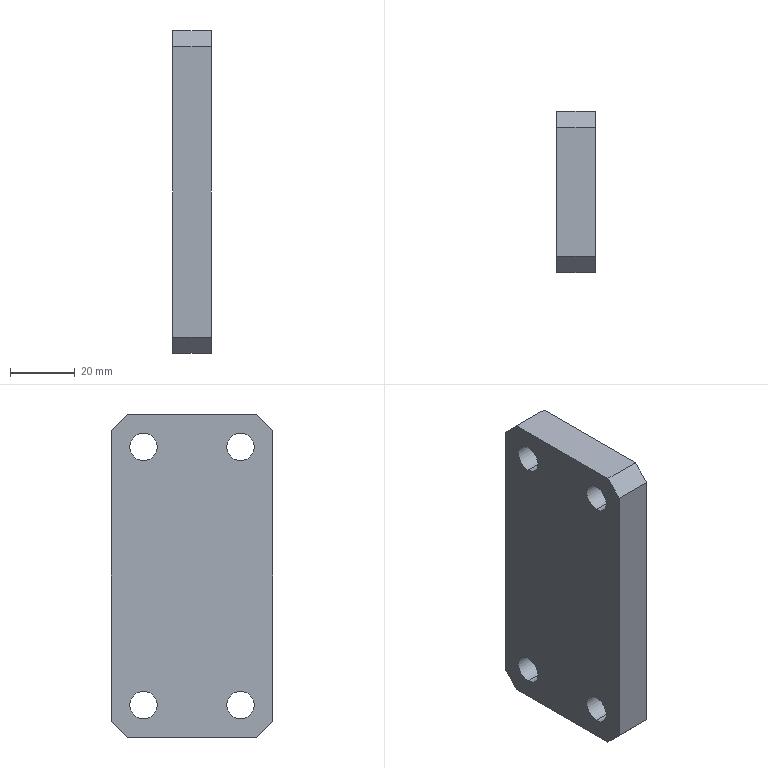Part | SolidWorks | features Chamfer 1, Extrusion 1, HoleWzd 1 | 1 solid | 18 faces | box 12 x 50 x 100 mm | volume 56676 mm3 | plane 10 | cylinder 8 | commonest cylinder face diameters 8.5 x8
STEP:
#1=CARTESIAN_POINT('',(0.,15.,44.25));
#2=VERTEX_POINT('',#1);
#3=CARTESIAN_POINT('',(0.,15.,35.75));
#4=VERTEX_POINT('',#3);
#5=CARTESIAN_POINT('',(0.,15.,40.));
#6=DIRECTION('',(1.,0.,0.));
#7=DIRECTION('',(0.,0.,-1.));
#8=AXIS2_PLACEMENT_3D('',#5,#6,#7);
#9=CIRCLE('',#8,4.25);
#10=EDGE_CURVE('',#2,#4,#9,.T.);
#11=ORIENTED_EDGE('',*,*,#10,.F.);
#12=CARTESIAN_POINT('',(12.,15.,44.25));
#13=VERTEX_POINT('',#12);
#14=CARTESIAN_POINT('',(12.,15.,44.25));
#15=DIRECTION('',(1.,0.,0.));
#16=VECTOR('',#15,1000.);
#17=LINE('',#14,#16);
#18=EDGE_CURVE('',#2,#13,#17,.T.);
#19=ORIENTED_EDGE('',*,*,#18,.T.);
#20=CARTESIAN_POINT('',(12.,15.,35.75));
#21=VERTEX_POINT('',#20);
#22=CARTESIAN_POINT('',(12.,15.,40.));
#23=DIRECTION('',(1.,0.,0.));
#24=DIRECTION('',(0.,0.,-1.));
#25=AXIS2_PLACEMENT_3D('',#22,#23,#24);
#26=CIRCLE('',#25,4.25);
#27=EDGE_CURVE('',#13,#21,#26,.T.);
#28=ORIENTED_EDGE('',*,*,#27,.T.);
#29=CARTESIAN_POINT('',(12.,15.,35.75));
#30=DIRECTION('',(1.,0.,0.));
#31=VECTOR('',#30,1000.);
#32=LINE('',#29,#31);
#33=EDGE_CURVE('',#4,#21,#32,.T.);
#34=ORIENTED_EDGE('',*,*,#33,.F.);
#35=EDGE_LOOP('',(#11,#19,#28,#34));
#36=FACE_OUTER_BOUND('',#35,.T.);
#37=CARTESIAN_POINT('',(12.,15.,40.));
#38=DIRECTION('',(1.,0.,0.));
#39=DIRECTION('',(0.,0.,-1.));
#40=AXIS2_PLACEMENT_3D('',#37,#38,#39);
#41=CYLINDRICAL_SURFACE('',#40,4.25);
#42=ADVANCED_FACE('',(#36),#41,.F.);
#43=CARTESIAN_POINT('',(0.,-15.,44.25));
#44=VERTEX_POINT('',#43);
#45=CARTESIAN_POINT('',(0.,-15.,35.75));
#46=VERTEX_POINT('',#45);
#47=CARTESIAN_POINT('',(0.,-15.,40.));
#48=DIRECTION('',(1.,0.,0.));
#49=DIRECTION('',(0.,0.,-1.));
#50=AXIS2_PLACEMENT_3D('',#47,#48,#49);
#51=CIRCLE('',#50,4.25);
#52=EDGE_CURVE('',#44,#46,#51,.T.);
#53=ORIENTED_EDGE('',*,*,#52,.F.);
#54=CARTESIAN_POINT('',(12.,-15.,44.25));
#55=VERTEX_POINT('',#54);
#56=CARTESIAN_POINT('',(12.,-15.,44.25));
#57=DIRECTION('',(1.,0.,0.));
#58=VECTOR('',#57,1000.);
#59=LINE('',#56,#58);
#60=EDGE_CURVE('',#44,#55,#59,.T.);
#61=ORIENTED_EDGE('',*,*,#60,.T.);
#62=CARTESIAN_POINT('',(12.,-15.,35.75));
#63=VERTEX_POINT('',#62);
#64=CARTESIAN_POINT('',(12.,-15.,40.));
#65=DIRECTION('',(1.,0.,0.));
#66=DIRECTION('',(0.,0.,-1.));
#67=AXIS2_PLACEMENT_3D('',#64,#65,#66);
#68=CIRCLE('',#67,4.25);
#69=EDGE_CURVE('',#55,#63,#68,.T.);
#70=ORIENTED_EDGE('',*,*,#69,.T.);
#71=CARTESIAN_POINT('',(12.,-15.,35.75));
#72=DIRECTION('',(1.,0.,0.));
#73=VECTOR('',#72,1000.);
#74=LINE('',#71,#73);
#75=EDGE_CURVE('',#46,#63,#74,.T.);
#76=ORIENTED_EDGE('',*,*,#75,.F.);
#77=EDGE_LOOP('',(#53,#61,#70,#76));
#78=FACE_OUTER_BOUND('',#77,.T.);
#79=CARTESIAN_POINT('',(12.,-15.,40.));
#80=DIRECTION('',(1.,0.,0.));
#81=DIRECTION('',(0.,0.,-1.));
#82=AXIS2_PLACEMENT_3D('',#79,#80,#81);
#83=CYLINDRICAL_SURFACE('',#82,4.25);
#84=ADVANCED_FACE('',(#78),#83,.F.);
#85=CARTESIAN_POINT('',(0.,15.,-35.75));
#86=VERTEX_POINT('',#85);
#87=CARTESIAN_POINT('',(0.,15.,-44.25));
#88=VERTEX_POINT('',#87);
#89=CARTESIAN_POINT('',(0.,15.,-40.));
#90=DIRECTION('',(1.,0.,0.));
#91=DIRECTION('',(0.,0.,-1.));
#92=AXIS2_PLACEMENT_3D('',#89,#90,#91);
#93=CIRCLE('',#92,4.25);
#94=EDGE_CURVE('',#86,#88,#93,.T.);
#95=ORIENTED_EDGE('',*,*,#94,.F.);
#96=CARTESIAN_POINT('',(12.,15.,-35.75));
#97=VERTEX_POINT('',#96);
#98=CARTESIAN_POINT('',(12.,15.,-35.75));
#99=DIRECTION('',(1.,0.,0.));
#100=VECTOR('',#99,1000.);
#101=LINE('',#98,#100);
#102=EDGE_CURVE('',#86,#97,#101,.T.);
#103=ORIENTED_EDGE('',*,*,#102,.T.);
#104=CARTESIAN_POINT('',(12.,15.,-44.25));
#105=VERTEX_POINT('',#104);
#106=CARTESIAN_POINT('',(12.,15.,-40.));
#107=DIRECTION('',(1.,0.,0.));
#108=DIRECTION('',(0.,0.,-1.));
#109=AXIS2_PLACEMENT_3D('',#106,#107,#108);
#110=CIRCLE('',#109,4.25);
#111=EDGE_CURVE('',#97,#105,#110,.T.);
#112=ORIENTED_EDGE('',*,*,#111,.T.);
#113=CARTESIAN_POINT('',(12.,15.,-44.25));
#114=DIRECTION('',(1.,0.,0.));
#115=VECTOR('',#114,1000.);
#116=LINE('',#113,#115);
#117=EDGE_CURVE('',#88,#105,#116,.T.);
#118=ORIENTED_EDGE('',*,*,#117,.F.);
#119=EDGE_LOOP('',(#95,#103,#112,#118));
#120=FACE_OUTER_BOUND('',#119,.T.);
#121=CARTESIAN_POINT('',(12.,15.,-40.));
#122=DIRECTION('',(1.,0.,0.));
#123=DIRECTION('',(0.,0.,-1.));
#124=AXIS2_PLACEMENT_3D('',#121,#122,#123);
#125=CYLINDRICAL_SURFACE('',#124,4.25);
#126=ADVANCED_FACE('',(#120),#125,.F.);
#127=CARTESIAN_POINT('',(0.,-15.,-35.75));
#128=VERTEX_POINT('',#127);
#129=CARTESIAN_POINT('',(0.,-15.,-44.25));
#130=VERTEX_POINT('',#129);
#131=CARTESIAN_POINT('',(0.,-15.,-40.));
#132=DIRECTION('',(1.,0.,0.));
#133=DIRECTION('',(0.,0.,-1.));
#134=AXIS2_PLACEMENT_3D('',#131,#132,#133);
#135=CIRCLE('',#134,4.25);
#136=EDGE_CURVE('',#128,#130,#135,.T.);
#137=ORIENTED_EDGE('',*,*,#136,.F.);
#138=CARTESIAN_POINT('',(12.,-15.,-35.75));
#139=VERTEX_POINT('',#138);
#140=CARTESIAN_POINT('',(12.,-15.,-35.75));
#141=DIRECTION('',(1.,0.,0.));
#142=VECTOR('',#141,1000.);
#143=LINE('',#140,#142);
#144=EDGE_CURVE('',#128,#139,#143,.T.);
#145=ORIENTED_EDGE('',*,*,#144,.T.);
#146=CARTESIAN_POINT('',(12.,-15.,-44.25));
#147=VERTEX_POINT('',#146);
#148=CARTESIAN_POINT('',(12.,-15.,-40.));
#149=DIRECTION('',(1.,0.,0.));
#150=DIRECTION('',(0.,0.,-1.));
#151=AXIS2_PLACEMENT_3D('',#148,#149,#150);
#152=CIRCLE('',#151,4.25);
#153=EDGE_CURVE('',#139,#147,#152,.T.);
#154=ORIENTED_EDGE('',*,*,#153,.T.);
#155=CARTESIAN_POINT('',(12.,-15.,-44.25));
#156=DIRECTION('',(1.,0.,0.));
#157=VECTOR('',#156,1000.);
#158=LINE('',#155,#157);
#159=EDGE_CURVE('',#130,#147,#158,.T.);
#160=ORIENTED_EDGE('',*,*,#159,.F.);
#161=EDGE_LOOP('',(#137,#145,#154,#160));
#162=FACE_OUTER_BOUND('',#161,.T.);
#163=CARTESIAN_POINT('',(12.,-15.,-40.));
#164=DIRECTION('',(1.,0.,0.));
#165=DIRECTION('',(0.,0.,-1.));
#166=AXIS2_PLACEMENT_3D('',#163,#164,#165);
#167=CYLINDRICAL_SURFACE('',#166,4.25);
#168=ADVANCED_FACE('',(#162),#167,.F.);
#169=CARTESIAN_POINT('',(0.,-20.,-50.));
#170=VERTEX_POINT('',#169);
#171=CARTESIAN_POINT('',(0.,20.,-50.));
#172=VERTEX_POINT('',#171);
#173=CARTESIAN_POINT('',(0.,25.,-50.));
#174=DIRECTION('',(0.,1.,0.));
#175=VECTOR('',#174,1000.);
#176=LINE('',#173,#175);
#177=EDGE_CURVE('',#170,#172,#176,.T.);
#178=ORIENTED_EDGE('',*,*,#177,.T.);
#179=CARTESIAN_POINT('',(12.,20.,-50.));
#180=VERTEX_POINT('',#179);
#181=CARTESIAN_POINT('',(12.,20.,-50.));
#182=DIRECTION('',(1.,0.,0.));
#183=VECTOR('',#182,1000.);
#184=LINE('',#181,#183);
#185=EDGE_CURVE('',#172,#180,#184,.T.);
#186=ORIENTED_EDGE('',*,*,#185,.T.);
#187=CARTESIAN_POINT('',(12.,-20.,-50.));
#188=VERTEX_POINT('',#187);
#189=CARTESIAN_POINT('',(12.,25.,-50.));
#190=DIRECTION('',(0.,1.,0.));
#191=VECTOR('',#190,1000.);
#192=LINE('',#189,#191);
#193=EDGE_CURVE('',#188,#180,#192,.T.);
#194=ORIENTED_EDGE('',*,*,#193,.F.);
#195=CARTESIAN_POINT('',(12.,-20.,-50.));
#196=DIRECTION('',(-1.,0.,0.));
#197=VECTOR('',#196,1000.);
#198=LINE('',#195,#197);
#199=EDGE_CURVE('',#188,#170,#198,.T.);
#200=ORIENTED_EDGE('',*,*,#199,.T.);
#201=EDGE_LOOP('',(#178,#186,#194,#200));
#202=FACE_OUTER_BOUND('',#201,.T.);
#203=CARTESIAN_POINT('',(12.,25.,-50.));
#204=DIRECTION('',(0.,0.,1.));
#205=DIRECTION('',(1.,0.,0.));
#206=AXIS2_PLACEMENT_3D('',#203,#204,#205);
#207=PLANE('',#206);
#208=ADVANCED_FACE('',(#202),#207,.F.);
#209=CARTESIAN_POINT('',(12.,25.,-45.));
#210=VERTEX_POINT('',#209);
#211=CARTESIAN_POINT('',(12.,25.,45.));
#212=VERTEX_POINT('',#211);
#213=CARTESIAN_POINT('',(12.,25.,50.));
#214=DIRECTION('',(0.,0.,1.));
#215=VECTOR('',#214,1000.);
#216=LINE('',#213,#215);
#217=EDGE_CURVE('',#210,#212,#216,.T.);
#218=ORIENTED_EDGE('',*,*,#217,.F.);
#219=CARTESIAN_POINT('',(0.,25.,-45.));
#220=VERTEX_POINT('',#219);
#221=CARTESIAN_POINT('',(12.,25.,-45.));
#222=DIRECTION('',(-1.,0.,0.));
#223=VECTOR('',#222,1000.);
#224=LINE('',#221,#223);
#225=EDGE_CURVE('',#210,#220,#224,.T.);
#226=ORIENTED_EDGE('',*,*,#225,.T.);
#227=CARTESIAN_POINT('',(0.,25.,45.));
#228=VERTEX_POINT('',#227);
#229=CARTESIAN_POINT('',(0.,25.,50.));
#230=DIRECTION('',(0.,0.,1.));
#231=VECTOR('',#230,1000.);
#232=LINE('',#229,#231);
#233=EDGE_CURVE('',#220,#228,#232,.T.);
#234=ORIENTED_EDGE('',*,*,#233,.T.);
#235=CARTESIAN_POINT('',(12.,25.,45.));
#236=DIRECTION('',(1.,0.,0.));
#237=VECTOR('',#236,1000.);
#238=LINE('',#235,#237);
#239=EDGE_CURVE('',#228,#212,#238,.T.);
#240=ORIENTED_EDGE('',*,*,#239,.T.);
#241=EDGE_LOOP('',(#218,#226,#234,#240));
#242=FACE_OUTER_BOUND('',#241,.T.);
#243=CARTESIAN_POINT('',(12.,25.,50.));
#244=DIRECTION('',(0.,-1.,0.));
#245=DIRECTION('',(0.,0.,-1.));
#246=AXIS2_PLACEMENT_3D('',#243,#244,#245);
#247=PLANE('',#246);
#248=ADVANCED_FACE('',(#242),#247,.F.);
#249=CARTESIAN_POINT('',(12.,20.,50.));
#250=VERTEX_POINT('',#249);
#251=CARTESIAN_POINT('',(12.,-20.,50.));
#252=VERTEX_POINT('',#251);
#253=CARTESIAN_POINT('',(12.,25.,50.));
#254=DIRECTION('',(0.,-1.,0.));
#255=VECTOR('',#254,1000.);
#256=LINE('',#253,#255);
#257=EDGE_CURVE('',#250,#252,#256,.T.);
#258=ORIENTED_EDGE('',*,*,#257,.F.);
#259=CARTESIAN_POINT('',(0.,20.,50.));
#260=VERTEX_POINT('',#259);
#261=CARTESIAN_POINT('',(12.,20.,50.));
#262=DIRECTION('',(-1.,0.,0.));
#263=VECTOR('',#262,1000.);
#264=LINE('',#261,#263);
#265=EDGE_CURVE('',#250,#260,#264,.T.);
#266=ORIENTED_EDGE('',*,*,#265,.T.);
#267=CARTESIAN_POINT('',(0.,-20.,50.));
#268=VERTEX_POINT('',#267);
#269=CARTESIAN_POINT('',(0.,25.,50.));
#270=DIRECTION('',(0.,-1.,0.));
#271=VECTOR('',#270,1000.);
#272=LINE('',#269,#271);
#273=EDGE_CURVE('',#260,#268,#272,.T.);
#274=ORIENTED_EDGE('',*,*,#273,.T.);
#275=CARTESIAN_POINT('',(12.,-20.,50.));
#276=DIRECTION('',(1.,0.,0.));
#277=VECTOR('',#276,1000.);
#278=LINE('',#275,#277);
#279=EDGE_CURVE('',#268,#252,#278,.T.);
#280=ORIENTED_EDGE('',*,*,#279,.T.);
#281=EDGE_LOOP('',(#258,#266,#274,#280));
#282=FACE_OUTER_BOUND('',#281,.T.);
#283=CARTESIAN_POINT('',(12.,25.,50.));
#284=DIRECTION('',(0.,0.,-1.));
#285=DIRECTION('',(0.,1.,0.));
#286=AXIS2_PLACEMENT_3D('',#283,#284,#285);
#287=PLANE('',#286);
#288=ADVANCED_FACE('',(#282),#287,.F.);
#289=CARTESIAN_POINT('',(0.,-25.,45.));
#290=VERTEX_POINT('',#289);
#291=CARTESIAN_POINT('',(0.,-25.,-45.));
#292=VERTEX_POINT('',#291);
#293=CARTESIAN_POINT('',(0.,-25.,50.));
#294=DIRECTION('',(0.,0.,-1.));
#295=VECTOR('',#294,1000.);
#296=LINE('',#293,#295);
#297=EDGE_CURVE('',#290,#292,#296,.T.);
#298=ORIENTED_EDGE('',*,*,#297,.T.);
#299=CARTESIAN_POINT('',(12.,-25.,-45.));
#300=VERTEX_POINT('',#299);
#301=CARTESIAN_POINT('',(12.,-25.,-45.));
#302=DIRECTION('',(1.,0.,0.));
#303=VECTOR('',#302,1000.);
#304=LINE('',#301,#303);
#305=EDGE_CURVE('',#292,#300,#304,.T.);
#306=ORIENTED_EDGE('',*,*,#305,.T.);
#307=CARTESIAN_POINT('',(12.,-25.,45.));
#308=VERTEX_POINT('',#307);
#309=CARTESIAN_POINT('',(12.,-25.,50.));
#310=DIRECTION('',(0.,0.,-1.));
#311=VECTOR('',#310,1000.);
#312=LINE('',#309,#311);
#313=EDGE_CURVE('',#308,#300,#312,.T.);
#314=ORIENTED_EDGE('',*,*,#313,.F.);
#315=CARTESIAN_POINT('',(12.,-25.,45.));
#316=DIRECTION('',(-1.,0.,0.));
#317=VECTOR('',#316,1000.);
#318=LINE('',#315,#317);
#319=EDGE_CURVE('',#308,#290,#318,.T.);
#320=ORIENTED_EDGE('',*,*,#319,.T.);
#321=EDGE_LOOP('',(#298,#306,#314,#320));
#322=FACE_OUTER_BOUND('',#321,.T.);
#323=CARTESIAN_POINT('',(12.,-25.,50.));
#324=DIRECTION('',(0.,1.,0.));
#325=DIRECTION('',(0.,0.,1.));
#326=AXIS2_PLACEMENT_3D('',#323,#324,#325);
#327=PLANE('',#326);
#328=ADVANCED_FACE('',(#322),#327,.F.);
#329=CARTESIAN_POINT('',(12.,15.,40.));
#330=DIRECTION('',(1.,0.,0.));
#331=DIRECTION('',(0.,0.,-1.));
#332=AXIS2_PLACEMENT_3D('',#329,#330,#331);
#333=CIRCLE('',#332,4.25);
#334=EDGE_CURVE('',#21,#13,#333,.T.);
#335=ORIENTED_EDGE('',*,*,#334,.F.);
#336=ORIENTED_EDGE('',*,*,#27,.F.);
#337=EDGE_LOOP('',(#335,#336));
#338=FACE_BOUND('',#337,.T.);
#339=CARTESIAN_POINT('',(12.,-15.,40.));
#340=DIRECTION('',(1.,0.,0.));
#341=DIRECTION('',(0.,0.,-1.));
#342=AXIS2_PLACEMENT_3D('',#339,#340,#341);
#343=CIRCLE('',#342,4.25);
#344=EDGE_CURVE('',#63,#55,#343,.T.);
#345=ORIENTED_EDGE('',*,*,#344,.F.);
#346=ORIENTED_EDGE('',*,*,#69,.F.);
#347=EDGE_LOOP('',(#345,#346));
#348=FACE_BOUND('',#347,.T.);
#349=CARTESIAN_POINT('',(12.,15.,-40.));
#350=DIRECTION('',(1.,0.,0.));
#351=DIRECTION('',(0.,0.,-1.));
#352=AXIS2_PLACEMENT_3D('',#349,#350,#351);
#353=CIRCLE('',#352,4.25);
#354=EDGE_CURVE('',#105,#97,#353,.T.);
#355=ORIENTED_EDGE('',*,*,#354,.F.);
#356=ORIENTED_EDGE('',*,*,#111,.F.);
#357=EDGE_LOOP('',(#355,#356));
#358=FACE_BOUND('',#357,.T.);
#359=CARTESIAN_POINT('',(12.,-15.,-40.));
#360=DIRECTION('',(1.,0.,0.));
#361=DIRECTION('',(0.,0.,-1.));
#362=AXIS2_PLACEMENT_3D('',#359,#360,#361);
#363=CIRCLE('',#362,4.25);
#364=EDGE_CURVE('',#147,#139,#363,.T.);
#365=ORIENTED_EDGE('',*,*,#364,.F.);
#366=ORIENTED_EDGE('',*,*,#153,.F.);
#367=EDGE_LOOP('',(#365,#366));
#368=FACE_BOUND('',#367,.T.);
#369=ORIENTED_EDGE('',*,*,#193,.T.);
#370=CARTESIAN_POINT('',(12.,35.,-35.));
#371=DIRECTION('',(0.,0.7071,0.7071));
#372=VECTOR('',#371,1000.);
#373=LINE('',#370,#372);
#374=EDGE_CURVE('',#180,#210,#373,.T.);
#375=ORIENTED_EDGE('',*,*,#374,.T.);
#376=ORIENTED_EDGE('',*,*,#217,.T.);
#377=CARTESIAN_POINT('',(12.,35.,35.));
#378=DIRECTION('',(0.,-0.7071,0.7071));
#379=VECTOR('',#378,1000.);
#380=LINE('',#377,#379);
#381=EDGE_CURVE('',#212,#250,#380,.T.);
#382=ORIENTED_EDGE('',*,*,#381,.T.);
#383=ORIENTED_EDGE('',*,*,#257,.T.);
#384=CARTESIAN_POINT('',(12.,-35.,35.));
#385=DIRECTION('',(0.,-0.7071,-0.7071));
#386=VECTOR('',#385,1000.);
#387=LINE('',#384,#386);
#388=EDGE_CURVE('',#252,#308,#387,.T.);
#389=ORIENTED_EDGE('',*,*,#388,.T.);
#390=ORIENTED_EDGE('',*,*,#313,.T.);
#391=CARTESIAN_POINT('',(12.,-35.,-35.));
#392=DIRECTION('',(0.,0.7071,-0.7071));
#393=VECTOR('',#392,1000.);
#394=LINE('',#391,#393);
#395=EDGE_CURVE('',#300,#188,#394,.T.);
#396=ORIENTED_EDGE('',*,*,#395,.T.);
#397=EDGE_LOOP('',(#369,#375,#376,#382,#383,#389,#390,#396));
#398=FACE_OUTER_BOUND('',#397,.T.);
#399=CARTESIAN_POINT('',(12.,0.,0.));
#400=DIRECTION('',(1.,0.,0.));
#401=DIRECTION('',(0.,0.,-1.));
#402=AXIS2_PLACEMENT_3D('',#399,#400,#401);
#403=PLANE('',#402);
#404=ADVANCED_FACE('',(#338,#348,#358,#368,#398),#403,.T.);
#405=CARTESIAN_POINT('',(0.,15.,40.));
#406=DIRECTION('',(1.,0.,0.));
#407=DIRECTION('',(0.,0.,-1.));
#408=AXIS2_PLACEMENT_3D('',#405,#406,#407);
#409=CIRCLE('',#408,4.25);
#410=EDGE_CURVE('',#4,#2,#409,.T.);
#411=ORIENTED_EDGE('',*,*,#410,.T.);
#412=ORIENTED_EDGE('',*,*,#10,.T.);
#413=EDGE_LOOP('',(#411,#412));
#414=FACE_BOUND('',#413,.T.);
#415=CARTESIAN_POINT('',(0.,-15.,40.));
#416=DIRECTION('',(1.,0.,0.));
#417=DIRECTION('',(0.,0.,-1.));
#418=AXIS2_PLACEMENT_3D('',#415,#416,#417);
#419=CIRCLE('',#418,4.25);
#420=EDGE_CURVE('',#46,#44,#419,.T.);
#421=ORIENTED_EDGE('',*,*,#420,.T.);
#422=ORIENTED_EDGE('',*,*,#52,.T.);
#423=EDGE_LOOP('',(#421,#422));
#424=FACE_BOUND('',#423,.T.);
#425=CARTESIAN_POINT('',(0.,15.,-40.));
#426=DIRECTION('',(1.,0.,0.));
#427=DIRECTION('',(0.,0.,-1.));
#428=AXIS2_PLACEMENT_3D('',#425,#426,#427);
#429=CIRCLE('',#428,4.25);
#430=EDGE_CURVE('',#88,#86,#429,.T.);
#431=ORIENTED_EDGE('',*,*,#430,.T.);
#432=ORIENTED_EDGE('',*,*,#94,.T.);
#433=EDGE_LOOP('',(#431,#432));
#434=FACE_BOUND('',#433,.T.);
#435=CARTESIAN_POINT('',(0.,-15.,-40.));
#436=DIRECTION('',(1.,0.,0.));
#437=DIRECTION('',(0.,0.,-1.));
#438=AXIS2_PLACEMENT_3D('',#435,#436,#437);
#439=CIRCLE('',#438,4.25);
#440=EDGE_CURVE('',#130,#128,#439,.T.);
#441=ORIENTED_EDGE('',*,*,#440,.T.);
#442=ORIENTED_EDGE('',*,*,#136,.T.);
#443=EDGE_LOOP('',(#441,#442));
#444=FACE_BOUND('',#443,.T.);
#445=ORIENTED_EDGE('',*,*,#233,.F.);
#446=CARTESIAN_POINT('',(0.,25.,-45.));
#447=DIRECTION('',(0.,-0.7071,-0.7071));
#448=VECTOR('',#447,1000.);
#449=LINE('',#446,#448);
#450=EDGE_CURVE('',#220,#172,#449,.T.);
#451=ORIENTED_EDGE('',*,*,#450,.T.);
#452=ORIENTED_EDGE('',*,*,#177,.F.);
#453=CARTESIAN_POINT('',(0.,-20.,-50.));
#454=DIRECTION('',(0.,-0.7071,0.7071));
#455=VECTOR('',#454,1000.);
#456=LINE('',#453,#455);
#457=EDGE_CURVE('',#170,#292,#456,.T.);
#458=ORIENTED_EDGE('',*,*,#457,.T.);
#459=ORIENTED_EDGE('',*,*,#297,.F.);
#460=CARTESIAN_POINT('',(0.,-25.,45.));
#461=DIRECTION('',(0.,0.7071,0.7071));
#462=VECTOR('',#461,1000.);
#463=LINE('',#460,#462);
#464=EDGE_CURVE('',#290,#268,#463,.T.);
#465=ORIENTED_EDGE('',*,*,#464,.T.);
#466=ORIENTED_EDGE('',*,*,#273,.F.);
#467=CARTESIAN_POINT('',(0.,20.,50.));
#468=DIRECTION('',(0.,0.7071,-0.7071));
#469=VECTOR('',#468,1000.);
#470=LINE('',#467,#469);
#471=EDGE_CURVE('',#260,#228,#470,.T.);
#472=ORIENTED_EDGE('',*,*,#471,.T.);
#473=EDGE_LOOP('',(#445,#451,#452,#458,#459,#465,#466,#472));
#474=FACE_OUTER_BOUND('',#473,.T.);
#475=CARTESIAN_POINT('',(0.,0.,0.));
#476=DIRECTION('',(1.,0.,0.));
#477=DIRECTION('',(0.,0.,-1.));
#478=AXIS2_PLACEMENT_3D('',#475,#476,#477);
#479=PLANE('',#478);
#480=ADVANCED_FACE('',(#414,#424,#434,#444,#474),#479,.F.);
#481=ORIENTED_EDGE('',*,*,#144,.F.);
#482=ORIENTED_EDGE('',*,*,#440,.F.);
#483=ORIENTED_EDGE('',*,*,#159,.T.);
#484=ORIENTED_EDGE('',*,*,#364,.T.);
#485=EDGE_LOOP('',(#481,#482,#483,#484));
#486=FACE_OUTER_BOUND('',#485,.T.);
#487=CARTESIAN_POINT('',(12.,-15.,-40.));
#488=DIRECTION('',(1.,0.,0.));
#489=DIRECTION('',(0.,0.,-1.));
#490=AXIS2_PLACEMENT_3D('',#487,#488,#489);
#491=CYLINDRICAL_SURFACE('',#490,4.25);
#492=ADVANCED_FACE('',(#486),#491,.F.);
#493=ORIENTED_EDGE('',*,*,#102,.F.);
#494=ORIENTED_EDGE('',*,*,#430,.F.);
#495=ORIENTED_EDGE('',*,*,#117,.T.);
#496=ORIENTED_EDGE('',*,*,#354,.T.);
#497=EDGE_LOOP('',(#493,#494,#495,#496));
#498=FACE_OUTER_BOUND('',#497,.T.);
#499=CARTESIAN_POINT('',(12.,15.,-40.));
#500=DIRECTION('',(1.,0.,0.));
#501=DIRECTION('',(0.,0.,-1.));
#502=AXIS2_PLACEMENT_3D('',#499,#500,#501);
#503=CYLINDRICAL_SURFACE('',#502,4.25);
#504=ADVANCED_FACE('',(#498),#503,.F.);
#505=ORIENTED_EDGE('',*,*,#60,.F.);
#506=ORIENTED_EDGE('',*,*,#420,.F.);
#507=ORIENTED_EDGE('',*,*,#75,.T.);
#508=ORIENTED_EDGE('',*,*,#344,.T.);
#509=EDGE_LOOP('',(#505,#506,#507,#508));
#510=FACE_OUTER_BOUND('',#509,.T.);
#511=CARTESIAN_POINT('',(12.,-15.,40.));
#512=DIRECTION('',(1.,0.,0.));
#513=DIRECTION('',(0.,0.,-1.));
#514=AXIS2_PLACEMENT_3D('',#511,#512,#513);
#515=CYLINDRICAL_SURFACE('',#514,4.25);
#516=ADVANCED_FACE('',(#510),#515,.F.);
#517=ORIENTED_EDGE('',*,*,#18,.F.);
#518=ORIENTED_EDGE('',*,*,#410,.F.);
#519=ORIENTED_EDGE('',*,*,#33,.T.);
#520=ORIENTED_EDGE('',*,*,#334,.T.);
#521=EDGE_LOOP('',(#517,#518,#519,#520));
#522=FACE_OUTER_BOUND('',#521,.T.);
#523=CARTESIAN_POINT('',(12.,15.,40.));
#524=DIRECTION('',(1.,0.,0.));
#525=DIRECTION('',(0.,0.,-1.));
#526=AXIS2_PLACEMENT_3D('',#523,#524,#525);
#527=CYLINDRICAL_SURFACE('',#526,4.25);
#528=ADVANCED_FACE('',(#522),#527,.F.);
#529=ORIENTED_EDGE('',*,*,#374,.F.);
#530=ORIENTED_EDGE('',*,*,#185,.F.);
#531=ORIENTED_EDGE('',*,*,#450,.F.);
#532=ORIENTED_EDGE('',*,*,#225,.F.);
#533=EDGE_LOOP('',(#529,#530,#531,#532));
#534=FACE_OUTER_BOUND('',#533,.T.);
#535=CARTESIAN_POINT('',(12.,25.,-45.));
#536=DIRECTION('',(0.,-0.7071,0.7071));
#537=DIRECTION('',(-1.,0.,0.));
#538=AXIS2_PLACEMENT_3D('',#535,#536,#537);
#539=PLANE('',#538);
#540=ADVANCED_FACE('',(#534),#539,.F.);
#541=ORIENTED_EDGE('',*,*,#395,.F.);
#542=ORIENTED_EDGE('',*,*,#305,.F.);
#543=ORIENTED_EDGE('',*,*,#457,.F.);
#544=ORIENTED_EDGE('',*,*,#199,.F.);
#545=EDGE_LOOP('',(#541,#542,#543,#544));
#546=FACE_OUTER_BOUND('',#545,.T.);
#547=CARTESIAN_POINT('',(12.,-20.,-50.));
#548=DIRECTION('',(0.,0.7071,0.7071));
#549=DIRECTION('',(-1.,0.,0.));
#550=AXIS2_PLACEMENT_3D('',#547,#548,#549);
#551=PLANE('',#550);
#552=ADVANCED_FACE('',(#546),#551,.F.);
#553=ORIENTED_EDGE('',*,*,#381,.F.);
#554=ORIENTED_EDGE('',*,*,#239,.F.);
#555=ORIENTED_EDGE('',*,*,#471,.F.);
#556=ORIENTED_EDGE('',*,*,#265,.F.);
#557=EDGE_LOOP('',(#553,#554,#555,#556));
#558=FACE_OUTER_BOUND('',#557,.T.);
#559=CARTESIAN_POINT('',(12.,20.,50.));
#560=DIRECTION('',(0.,-0.7071,-0.7071));
#561=DIRECTION('',(-1.,0.,0.));
#562=AXIS2_PLACEMENT_3D('',#559,#560,#561);
#563=PLANE('',#562);
#564=ADVANCED_FACE('',(#558),#563,.F.);
#565=ORIENTED_EDGE('',*,*,#388,.F.);
#566=ORIENTED_EDGE('',*,*,#279,.F.);
#567=ORIENTED_EDGE('',*,*,#464,.F.);
#568=ORIENTED_EDGE('',*,*,#319,.F.);
#569=EDGE_LOOP('',(#565,#566,#567,#568));
#570=FACE_OUTER_BOUND('',#569,.T.);
#571=CARTESIAN_POINT('',(12.,-25.,45.));
#572=DIRECTION('',(0.,0.7071,-0.7071));
#573=DIRECTION('',(-1.,0.,0.));
#574=AXIS2_PLACEMENT_3D('',#571,#572,#573);
#575=PLANE('',#574);
#576=ADVANCED_FACE('',(#570),#575,.F.);
#577=CLOSED_SHELL('',(#42,#84,#126,#168,#208,#248,#288,#328,#404,#480,#492,#504,#516,#528,#540,#552,#564,#576));
#578=MANIFOLD_SOLID_BREP('',#577);
#579=CARTESIAN_POINT('',(0.,0.,0.));
#580=DIRECTION('',(0.,0.,1.));
#581=DIRECTION('',(1.,0.,0.));
#582=AXIS2_PLACEMENT_3D('',#579,#580,#581);
#583=(LENGTH_UNIT()NAMED_UNIT(*)SI_UNIT(.MILLI.,.METRE.));
#584=UNCERTAINTY_MEASURE_WITH_UNIT(LENGTH_MEASURE(0.00001),#583,'','');
#585=(NAMED_UNIT(*)PLANE_ANGLE_UNIT()SI_UNIT($,.RADIAN.));
#586=(NAMED_UNIT(*)SI_UNIT($,.STERADIAN.)SOLID_ANGLE_UNIT());
#587=(GEOMETRIC_REPRESENTATION_CONTEXT(3)GLOBAL_UNCERTAINTY_ASSIGNED_CONTEXT((#584))GLOBAL_UNIT_ASSIGNED_CONTEXT((#583,#585,#586))REPRESENTATION_CONTEXT('',''));
#588=ADVANCED_BREP_SHAPE_REPRESENTATION('',(#578,#582),#587);